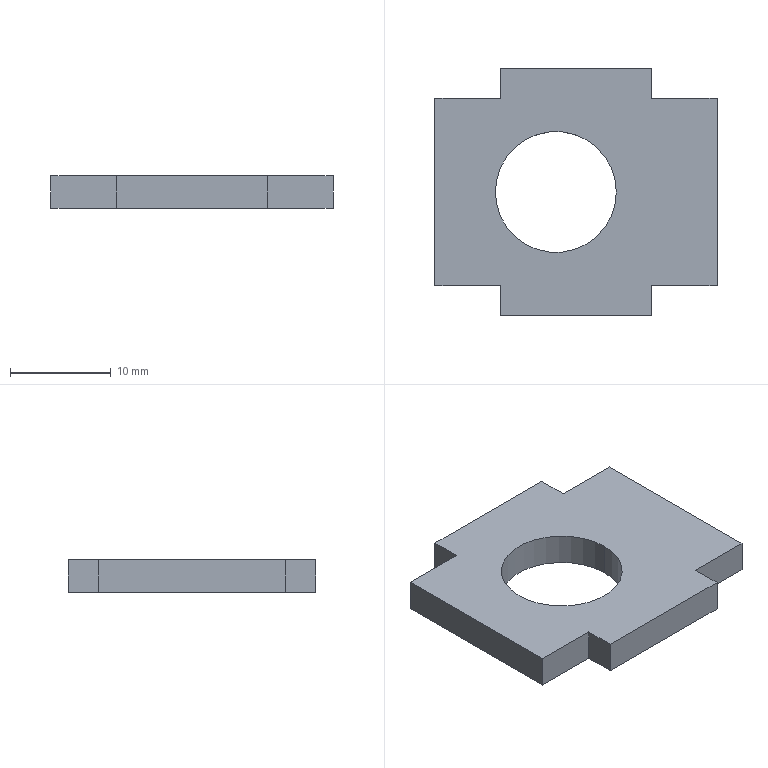Part | SolidWorks | features FlatPattern 1, SMBaseFlange 1, SheetMetal 1 | 1 solid | 16 faces | box 28 x 24.6 x 3.2 mm | volume 1593 mm3 | plane 14 | cylinder 2 | commonest cylinder face diameters 12 x2
STEP:
#1=CARTESIAN_POINT('',(213.,12.5,-3.2));
#2=VERTEX_POINT('',#1);
#3=CARTESIAN_POINT('',(225.,12.5,-3.2));
#4=VERTEX_POINT('',#3);
#5=CARTESIAN_POINT('',(219.,12.5,-3.2));
#6=DIRECTION('',(0.,0.,1.));
#7=DIRECTION('',(1.,0.,0.));
#8=AXIS2_PLACEMENT_3D('',#5,#6,#7);
#9=CIRCLE('',#8,6.);
#10=EDGE_CURVE('',#2,#4,#9,.T.);
#11=ORIENTED_EDGE('',*,*,#10,.F.);
#12=CARTESIAN_POINT('',(213.,12.5,0.));
#13=VERTEX_POINT('',#12);
#14=CARTESIAN_POINT('',(213.,12.5,-3.2));
#15=DIRECTION('',(0.,0.,1.));
#16=VECTOR('',#15,1000.);
#17=LINE('',#14,#16);
#18=EDGE_CURVE('',#2,#13,#17,.T.);
#19=ORIENTED_EDGE('',*,*,#18,.T.);
#20=CARTESIAN_POINT('',(225.,12.5,0.));
#21=VERTEX_POINT('',#20);
#22=CARTESIAN_POINT('',(219.,12.5,0.));
#23=DIRECTION('',(0.,0.,1.));
#24=DIRECTION('',(1.,0.,0.));
#25=AXIS2_PLACEMENT_3D('',#22,#23,#24);
#26=CIRCLE('',#25,6.);
#27=EDGE_CURVE('',#13,#21,#26,.T.);
#28=ORIENTED_EDGE('',*,*,#27,.T.);
#29=CARTESIAN_POINT('',(225.,12.5,-3.2));
#30=DIRECTION('',(0.,0.,1.));
#31=VECTOR('',#30,1000.);
#32=LINE('',#29,#31);
#33=EDGE_CURVE('',#4,#21,#32,.T.);
#34=ORIENTED_EDGE('',*,*,#33,.F.);
#35=EDGE_LOOP('',(#11,#19,#28,#34));
#36=FACE_OUTER_BOUND('',#35,.T.);
#37=CARTESIAN_POINT('',(219.,12.5,-3.2));
#38=DIRECTION('',(0.,0.,1.));
#39=DIRECTION('',(1.,0.,0.));
#40=AXIS2_PLACEMENT_3D('',#37,#38,#39);
#41=CYLINDRICAL_SURFACE('',#40,6.);
#42=ADVANCED_FACE('',(#36),#41,.F.);
#43=CARTESIAN_POINT('',(207.,21.8,0.));
#44=VERTEX_POINT('',#43);
#45=CARTESIAN_POINT('',(207.,3.2,0.));
#46=VERTEX_POINT('',#45);
#47=CARTESIAN_POINT('',(207.,3.2,0.));
#48=DIRECTION('',(0.,-1.,0.));
#49=VECTOR('',#48,1000.);
#50=LINE('',#47,#49);
#51=EDGE_CURVE('',#44,#46,#50,.T.);
#52=ORIENTED_EDGE('',*,*,#51,.F.);
#53=CARTESIAN_POINT('',(207.,21.8,-3.2));
#54=VERTEX_POINT('',#53);
#55=CARTESIAN_POINT('',(207.,21.8,-3.2));
#56=DIRECTION('',(0.,0.,1.));
#57=VECTOR('',#56,1000.);
#58=LINE('',#55,#57);
#59=EDGE_CURVE('',#54,#44,#58,.T.);
#60=ORIENTED_EDGE('',*,*,#59,.F.);
#61=CARTESIAN_POINT('',(207.,3.2,-3.2));
#62=VERTEX_POINT('',#61);
#63=CARTESIAN_POINT('',(207.,3.2,-3.2));
#64=DIRECTION('',(0.,-1.,0.));
#65=VECTOR('',#64,1000.);
#66=LINE('',#63,#65);
#67=EDGE_CURVE('',#54,#62,#66,.T.);
#68=ORIENTED_EDGE('',*,*,#67,.T.);
#69=CARTESIAN_POINT('',(207.,3.2,-3.2));
#70=DIRECTION('',(0.,0.,1.));
#71=VECTOR('',#70,1000.);
#72=LINE('',#69,#71);
#73=EDGE_CURVE('',#62,#46,#72,.T.);
#74=ORIENTED_EDGE('',*,*,#73,.T.);
#75=EDGE_LOOP('',(#52,#60,#68,#74));
#76=FACE_OUTER_BOUND('',#75,.T.);
#77=CARTESIAN_POINT('',(207.,3.2,-3.2));
#78=DIRECTION('',(-1.,0.,0.));
#79=DIRECTION('',(0.,0.,1.));
#80=AXIS2_PLACEMENT_3D('',#77,#78,#79);
#81=PLANE('',#80);
#82=ADVANCED_FACE('',(#76),#81,.T.);
#83=CARTESIAN_POINT('',(213.5,21.8,0.));
#84=VERTEX_POINT('',#83);
#85=CARTESIAN_POINT('',(207.,21.8,0.));
#86=DIRECTION('',(-1.,0.,0.));
#87=VECTOR('',#86,1000.);
#88=LINE('',#85,#87);
#89=EDGE_CURVE('',#84,#44,#88,.T.);
#90=ORIENTED_EDGE('',*,*,#89,.F.);
#91=CARTESIAN_POINT('',(213.5,21.8,-3.2));
#92=VERTEX_POINT('',#91);
#93=CARTESIAN_POINT('',(213.5,21.8,-3.2));
#94=DIRECTION('',(0.,0.,1.));
#95=VECTOR('',#94,1000.);
#96=LINE('',#93,#95);
#97=EDGE_CURVE('',#92,#84,#96,.T.);
#98=ORIENTED_EDGE('',*,*,#97,.F.);
#99=CARTESIAN_POINT('',(207.,21.8,-3.2));
#100=DIRECTION('',(-1.,0.,0.));
#101=VECTOR('',#100,1000.);
#102=LINE('',#99,#101);
#103=EDGE_CURVE('',#92,#54,#102,.T.);
#104=ORIENTED_EDGE('',*,*,#103,.T.);
#105=ORIENTED_EDGE('',*,*,#59,.T.);
#106=EDGE_LOOP('',(#90,#98,#104,#105));
#107=FACE_OUTER_BOUND('',#106,.T.);
#108=CARTESIAN_POINT('',(207.,21.8,-3.2));
#109=DIRECTION('',(0.,1.,0.));
#110=DIRECTION('',(0.,0.,1.));
#111=AXIS2_PLACEMENT_3D('',#108,#109,#110);
#112=PLANE('',#111);
#113=ADVANCED_FACE('',(#107),#112,.T.);
#114=CARTESIAN_POINT('',(213.5,24.8,0.));
#115=VERTEX_POINT('',#114);
#116=CARTESIAN_POINT('',(213.5,21.8,0.));
#117=DIRECTION('',(0.,-1.,0.));
#118=VECTOR('',#117,1000.);
#119=LINE('',#116,#118);
#120=EDGE_CURVE('',#115,#84,#119,.T.);
#121=ORIENTED_EDGE('',*,*,#120,.F.);
#122=CARTESIAN_POINT('',(213.5,24.8,-3.2));
#123=VERTEX_POINT('',#122);
#124=CARTESIAN_POINT('',(213.5,24.8,-3.2));
#125=DIRECTION('',(0.,0.,1.));
#126=VECTOR('',#125,1000.);
#127=LINE('',#124,#126);
#128=EDGE_CURVE('',#123,#115,#127,.T.);
#129=ORIENTED_EDGE('',*,*,#128,.F.);
#130=CARTESIAN_POINT('',(213.5,21.8,-3.2));
#131=DIRECTION('',(0.,-1.,0.));
#132=VECTOR('',#131,1000.);
#133=LINE('',#130,#132);
#134=EDGE_CURVE('',#123,#92,#133,.T.);
#135=ORIENTED_EDGE('',*,*,#134,.T.);
#136=ORIENTED_EDGE('',*,*,#97,.T.);
#137=EDGE_LOOP('',(#121,#129,#135,#136));
#138=FACE_OUTER_BOUND('',#137,.T.);
#139=CARTESIAN_POINT('',(213.5,21.8,-3.2));
#140=DIRECTION('',(-1.,0.,0.));
#141=DIRECTION('',(0.,0.,1.));
#142=AXIS2_PLACEMENT_3D('',#139,#140,#141);
#143=PLANE('',#142);
#144=ADVANCED_FACE('',(#138),#143,.T.);
#145=CARTESIAN_POINT('',(228.5,24.8,0.));
#146=VERTEX_POINT('',#145);
#147=CARTESIAN_POINT('',(213.5,24.8,0.));
#148=DIRECTION('',(-1.,0.,0.));
#149=VECTOR('',#148,1000.);
#150=LINE('',#147,#149);
#151=EDGE_CURVE('',#146,#115,#150,.T.);
#152=ORIENTED_EDGE('',*,*,#151,.F.);
#153=CARTESIAN_POINT('',(228.5,24.8,-3.2));
#154=VERTEX_POINT('',#153);
#155=CARTESIAN_POINT('',(228.5,24.8,-3.2));
#156=DIRECTION('',(0.,0.,1.));
#157=VECTOR('',#156,1000.);
#158=LINE('',#155,#157);
#159=EDGE_CURVE('',#154,#146,#158,.T.);
#160=ORIENTED_EDGE('',*,*,#159,.F.);
#161=CARTESIAN_POINT('',(213.5,24.8,-3.2));
#162=DIRECTION('',(-1.,0.,0.));
#163=VECTOR('',#162,1000.);
#164=LINE('',#161,#163);
#165=EDGE_CURVE('',#154,#123,#164,.T.);
#166=ORIENTED_EDGE('',*,*,#165,.T.);
#167=ORIENTED_EDGE('',*,*,#128,.T.);
#168=EDGE_LOOP('',(#152,#160,#166,#167));
#169=FACE_OUTER_BOUND('',#168,.T.);
#170=CARTESIAN_POINT('',(213.5,24.8,-3.2));
#171=DIRECTION('',(0.,1.,0.));
#172=DIRECTION('',(0.,0.,1.));
#173=AXIS2_PLACEMENT_3D('',#170,#171,#172);
#174=PLANE('',#173);
#175=ADVANCED_FACE('',(#169),#174,.T.);
#176=CARTESIAN_POINT('',(228.5,21.8,0.));
#177=VERTEX_POINT('',#176);
#178=CARTESIAN_POINT('',(228.5,24.8,0.));
#179=DIRECTION('',(0.,1.,0.));
#180=VECTOR('',#179,1000.);
#181=LINE('',#178,#180);
#182=EDGE_CURVE('',#177,#146,#181,.T.);
#183=ORIENTED_EDGE('',*,*,#182,.F.);
#184=CARTESIAN_POINT('',(228.5,21.8,-3.2));
#185=VERTEX_POINT('',#184);
#186=CARTESIAN_POINT('',(228.5,21.8,-3.2));
#187=DIRECTION('',(0.,0.,1.));
#188=VECTOR('',#187,1000.);
#189=LINE('',#186,#188);
#190=EDGE_CURVE('',#185,#177,#189,.T.);
#191=ORIENTED_EDGE('',*,*,#190,.F.);
#192=CARTESIAN_POINT('',(228.5,24.8,-3.2));
#193=DIRECTION('',(0.,1.,0.));
#194=VECTOR('',#193,1000.);
#195=LINE('',#192,#194);
#196=EDGE_CURVE('',#185,#154,#195,.T.);
#197=ORIENTED_EDGE('',*,*,#196,.T.);
#198=ORIENTED_EDGE('',*,*,#159,.T.);
#199=EDGE_LOOP('',(#183,#191,#197,#198));
#200=FACE_OUTER_BOUND('',#199,.T.);
#201=CARTESIAN_POINT('',(228.5,24.8,-3.2));
#202=DIRECTION('',(1.,0.,0.));
#203=DIRECTION('',(0.,0.,-1.));
#204=AXIS2_PLACEMENT_3D('',#201,#202,#203);
#205=PLANE('',#204);
#206=ADVANCED_FACE('',(#200),#205,.T.);
#207=CARTESIAN_POINT('',(235.,21.8,0.));
#208=VERTEX_POINT('',#207);
#209=CARTESIAN_POINT('',(228.5,21.8,0.));
#210=DIRECTION('',(-1.,0.,0.));
#211=VECTOR('',#210,1000.);
#212=LINE('',#209,#211);
#213=EDGE_CURVE('',#208,#177,#212,.T.);
#214=ORIENTED_EDGE('',*,*,#213,.F.);
#215=CARTESIAN_POINT('',(235.,21.8,-3.2));
#216=VERTEX_POINT('',#215);
#217=CARTESIAN_POINT('',(235.,21.8,-3.2));
#218=DIRECTION('',(0.,0.,1.));
#219=VECTOR('',#218,1000.);
#220=LINE('',#217,#219);
#221=EDGE_CURVE('',#216,#208,#220,.T.);
#222=ORIENTED_EDGE('',*,*,#221,.F.);
#223=CARTESIAN_POINT('',(228.5,21.8,-3.2));
#224=DIRECTION('',(-1.,0.,0.));
#225=VECTOR('',#224,1000.);
#226=LINE('',#223,#225);
#227=EDGE_CURVE('',#216,#185,#226,.T.);
#228=ORIENTED_EDGE('',*,*,#227,.T.);
#229=ORIENTED_EDGE('',*,*,#190,.T.);
#230=EDGE_LOOP('',(#214,#222,#228,#229));
#231=FACE_OUTER_BOUND('',#230,.T.);
#232=CARTESIAN_POINT('',(228.5,21.8,-3.2));
#233=DIRECTION('',(0.,1.,0.));
#234=DIRECTION('',(0.,0.,1.));
#235=AXIS2_PLACEMENT_3D('',#232,#233,#234);
#236=PLANE('',#235);
#237=ADVANCED_FACE('',(#231),#236,.T.);
#238=CARTESIAN_POINT('',(235.,3.2,0.));
#239=VERTEX_POINT('',#238);
#240=CARTESIAN_POINT('',(235.,3.2,0.));
#241=DIRECTION('',(0.,1.,0.));
#242=VECTOR('',#241,1000.);
#243=LINE('',#240,#242);
#244=EDGE_CURVE('',#239,#208,#243,.T.);
#245=ORIENTED_EDGE('',*,*,#244,.F.);
#246=CARTESIAN_POINT('',(235.,3.2,-3.2));
#247=VERTEX_POINT('',#246);
#248=CARTESIAN_POINT('',(235.,3.2,-3.2));
#249=DIRECTION('',(0.,0.,1.));
#250=VECTOR('',#249,1000.);
#251=LINE('',#248,#250);
#252=EDGE_CURVE('',#247,#239,#251,.T.);
#253=ORIENTED_EDGE('',*,*,#252,.F.);
#254=CARTESIAN_POINT('',(235.,3.2,-3.2));
#255=DIRECTION('',(0.,1.,0.));
#256=VECTOR('',#255,1000.);
#257=LINE('',#254,#256);
#258=EDGE_CURVE('',#247,#216,#257,.T.);
#259=ORIENTED_EDGE('',*,*,#258,.T.);
#260=ORIENTED_EDGE('',*,*,#221,.T.);
#261=EDGE_LOOP('',(#245,#253,#259,#260));
#262=FACE_OUTER_BOUND('',#261,.T.);
#263=CARTESIAN_POINT('',(235.,3.2,-3.2));
#264=DIRECTION('',(1.,0.,0.));
#265=DIRECTION('',(0.,0.,-1.));
#266=AXIS2_PLACEMENT_3D('',#263,#264,#265);
#267=PLANE('',#266);
#268=ADVANCED_FACE('',(#262),#267,.T.);
#269=CARTESIAN_POINT('',(228.5,3.2,0.));
#270=VERTEX_POINT('',#269);
#271=CARTESIAN_POINT('',(228.5,3.2,0.));
#272=DIRECTION('',(1.,0.,0.));
#273=VECTOR('',#272,1000.);
#274=LINE('',#271,#273);
#275=EDGE_CURVE('',#270,#239,#274,.T.);
#276=ORIENTED_EDGE('',*,*,#275,.F.);
#277=CARTESIAN_POINT('',(228.5,3.2,-3.2));
#278=VERTEX_POINT('',#277);
#279=CARTESIAN_POINT('',(228.5,3.2,-3.2));
#280=DIRECTION('',(0.,0.,1.));
#281=VECTOR('',#280,1000.);
#282=LINE('',#279,#281);
#283=EDGE_CURVE('',#278,#270,#282,.T.);
#284=ORIENTED_EDGE('',*,*,#283,.F.);
#285=CARTESIAN_POINT('',(228.5,3.2,-3.2));
#286=DIRECTION('',(1.,0.,0.));
#287=VECTOR('',#286,1000.);
#288=LINE('',#285,#287);
#289=EDGE_CURVE('',#278,#247,#288,.T.);
#290=ORIENTED_EDGE('',*,*,#289,.T.);
#291=ORIENTED_EDGE('',*,*,#252,.T.);
#292=EDGE_LOOP('',(#276,#284,#290,#291));
#293=FACE_OUTER_BOUND('',#292,.T.);
#294=CARTESIAN_POINT('',(228.5,3.2,-3.2));
#295=DIRECTION('',(0.,-1.,0.));
#296=DIRECTION('',(0.,0.,-1.));
#297=AXIS2_PLACEMENT_3D('',#294,#295,#296);
#298=PLANE('',#297);
#299=ADVANCED_FACE('',(#293),#298,.T.);
#300=CARTESIAN_POINT('',(228.5,0.2,0.));
#301=VERTEX_POINT('',#300);
#302=CARTESIAN_POINT('',(228.5,0.2,0.));
#303=DIRECTION('',(0.,1.,0.));
#304=VECTOR('',#303,1000.);
#305=LINE('',#302,#304);
#306=EDGE_CURVE('',#301,#270,#305,.T.);
#307=ORIENTED_EDGE('',*,*,#306,.F.);
#308=CARTESIAN_POINT('',(228.5,0.2,-3.2));
#309=VERTEX_POINT('',#308);
#310=CARTESIAN_POINT('',(228.5,0.2,-3.2));
#311=DIRECTION('',(0.,0.,1.));
#312=VECTOR('',#311,1000.);
#313=LINE('',#310,#312);
#314=EDGE_CURVE('',#309,#301,#313,.T.);
#315=ORIENTED_EDGE('',*,*,#314,.F.);
#316=CARTESIAN_POINT('',(228.5,0.2,-3.2));
#317=DIRECTION('',(0.,1.,0.));
#318=VECTOR('',#317,1000.);
#319=LINE('',#316,#318);
#320=EDGE_CURVE('',#309,#278,#319,.T.);
#321=ORIENTED_EDGE('',*,*,#320,.T.);
#322=ORIENTED_EDGE('',*,*,#283,.T.);
#323=EDGE_LOOP('',(#307,#315,#321,#322));
#324=FACE_OUTER_BOUND('',#323,.T.);
#325=CARTESIAN_POINT('',(228.5,0.2,-3.2));
#326=DIRECTION('',(1.,0.,0.));
#327=DIRECTION('',(0.,0.,-1.));
#328=AXIS2_PLACEMENT_3D('',#325,#326,#327);
#329=PLANE('',#328);
#330=ADVANCED_FACE('',(#324),#329,.T.);
#331=CARTESIAN_POINT('',(213.5,0.2,0.));
#332=VERTEX_POINT('',#331);
#333=CARTESIAN_POINT('',(213.5,0.2,0.));
#334=DIRECTION('',(1.,0.,0.));
#335=VECTOR('',#334,1000.);
#336=LINE('',#333,#335);
#337=EDGE_CURVE('',#332,#301,#336,.T.);
#338=ORIENTED_EDGE('',*,*,#337,.F.);
#339=CARTESIAN_POINT('',(213.5,0.2,-3.2));
#340=VERTEX_POINT('',#339);
#341=CARTESIAN_POINT('',(213.5,0.2,-3.2));
#342=DIRECTION('',(0.,0.,1.));
#343=VECTOR('',#342,1000.);
#344=LINE('',#341,#343);
#345=EDGE_CURVE('',#340,#332,#344,.T.);
#346=ORIENTED_EDGE('',*,*,#345,.F.);
#347=CARTESIAN_POINT('',(213.5,0.2,-3.2));
#348=DIRECTION('',(1.,0.,0.));
#349=VECTOR('',#348,1000.);
#350=LINE('',#347,#349);
#351=EDGE_CURVE('',#340,#309,#350,.T.);
#352=ORIENTED_EDGE('',*,*,#351,.T.);
#353=ORIENTED_EDGE('',*,*,#314,.T.);
#354=EDGE_LOOP('',(#338,#346,#352,#353));
#355=FACE_OUTER_BOUND('',#354,.T.);
#356=CARTESIAN_POINT('',(213.5,0.2,-3.2));
#357=DIRECTION('',(0.,-1.,0.));
#358=DIRECTION('',(0.,0.,-1.));
#359=AXIS2_PLACEMENT_3D('',#356,#357,#358);
#360=PLANE('',#359);
#361=ADVANCED_FACE('',(#355),#360,.T.);
#362=CARTESIAN_POINT('',(213.5,3.2,0.));
#363=VERTEX_POINT('',#362);
#364=CARTESIAN_POINT('',(213.5,3.2,0.));
#365=DIRECTION('',(0.,-1.,0.));
#366=VECTOR('',#365,1000.);
#367=LINE('',#364,#366);
#368=EDGE_CURVE('',#363,#332,#367,.T.);
#369=ORIENTED_EDGE('',*,*,#368,.F.);
#370=CARTESIAN_POINT('',(213.5,3.2,-3.2));
#371=VERTEX_POINT('',#370);
#372=CARTESIAN_POINT('',(213.5,3.2,-3.2));
#373=DIRECTION('',(0.,0.,1.));
#374=VECTOR('',#373,1000.);
#375=LINE('',#372,#374);
#376=EDGE_CURVE('',#371,#363,#375,.T.);
#377=ORIENTED_EDGE('',*,*,#376,.F.);
#378=CARTESIAN_POINT('',(213.5,3.2,-3.2));
#379=DIRECTION('',(0.,-1.,0.));
#380=VECTOR('',#379,1000.);
#381=LINE('',#378,#380);
#382=EDGE_CURVE('',#371,#340,#381,.T.);
#383=ORIENTED_EDGE('',*,*,#382,.T.);
#384=ORIENTED_EDGE('',*,*,#345,.T.);
#385=EDGE_LOOP('',(#369,#377,#383,#384));
#386=FACE_OUTER_BOUND('',#385,.T.);
#387=CARTESIAN_POINT('',(213.5,3.2,-3.2));
#388=DIRECTION('',(-1.,0.,0.));
#389=DIRECTION('',(0.,0.,1.));
#390=AXIS2_PLACEMENT_3D('',#387,#388,#389);
#391=PLANE('',#390);
#392=ADVANCED_FACE('',(#386),#391,.T.);
#393=CARTESIAN_POINT('',(207.,3.2,0.));
#394=DIRECTION('',(1.,0.,0.));
#395=VECTOR('',#394,1000.);
#396=LINE('',#393,#395);
#397=EDGE_CURVE('',#46,#363,#396,.T.);
#398=ORIENTED_EDGE('',*,*,#397,.F.);
#399=ORIENTED_EDGE('',*,*,#73,.F.);
#400=CARTESIAN_POINT('',(207.,3.2,-3.2));
#401=DIRECTION('',(1.,0.,0.));
#402=VECTOR('',#401,1000.);
#403=LINE('',#400,#402);
#404=EDGE_CURVE('',#62,#371,#403,.T.);
#405=ORIENTED_EDGE('',*,*,#404,.T.);
#406=ORIENTED_EDGE('',*,*,#376,.T.);
#407=EDGE_LOOP('',(#398,#399,#405,#406));
#408=FACE_OUTER_BOUND('',#407,.T.);
#409=CARTESIAN_POINT('',(207.,3.2,-3.2));
#410=DIRECTION('',(0.,-1.,0.));
#411=DIRECTION('',(1.,0.,0.));
#412=AXIS2_PLACEMENT_3D('',#409,#410,#411);
#413=PLANE('',#412);
#414=ADVANCED_FACE('',(#408),#413,.T.);
#415=CARTESIAN_POINT('',(219.,12.5,-3.2));
#416=DIRECTION('',(0.,0.,1.));
#417=DIRECTION('',(1.,0.,0.));
#418=AXIS2_PLACEMENT_3D('',#415,#416,#417);
#419=CIRCLE('',#418,6.);
#420=EDGE_CURVE('',#4,#2,#419,.T.);
#421=ORIENTED_EDGE('',*,*,#420,.T.);
#422=ORIENTED_EDGE('',*,*,#10,.T.);
#423=EDGE_LOOP('',(#421,#422));
#424=FACE_BOUND('',#423,.T.);
#425=ORIENTED_EDGE('',*,*,#67,.F.);
#426=ORIENTED_EDGE('',*,*,#103,.F.);
#427=ORIENTED_EDGE('',*,*,#134,.F.);
#428=ORIENTED_EDGE('',*,*,#165,.F.);
#429=ORIENTED_EDGE('',*,*,#196,.F.);
#430=ORIENTED_EDGE('',*,*,#227,.F.);
#431=ORIENTED_EDGE('',*,*,#258,.F.);
#432=ORIENTED_EDGE('',*,*,#289,.F.);
#433=ORIENTED_EDGE('',*,*,#320,.F.);
#434=ORIENTED_EDGE('',*,*,#351,.F.);
#435=ORIENTED_EDGE('',*,*,#382,.F.);
#436=ORIENTED_EDGE('',*,*,#404,.F.);
#437=EDGE_LOOP('',(#425,#426,#427,#428,#429,#430,#431,#432,#433,#434,#435,#436));
#438=FACE_OUTER_BOUND('',#437,.T.);
#439=CARTESIAN_POINT('',(0.,0.,-3.2));
#440=DIRECTION('',(0.,0.,-1.));
#441=DIRECTION('',(-1.,0.,0.));
#442=AXIS2_PLACEMENT_3D('',#439,#440,#441);
#443=PLANE('',#442);
#444=ADVANCED_FACE('',(#424,#438),#443,.T.);
#445=CARTESIAN_POINT('',(219.,12.5,0.));
#446=DIRECTION('',(0.,0.,1.));
#447=DIRECTION('',(1.,0.,0.));
#448=AXIS2_PLACEMENT_3D('',#445,#446,#447);
#449=CIRCLE('',#448,6.);
#450=EDGE_CURVE('',#21,#13,#449,.T.);
#451=ORIENTED_EDGE('',*,*,#450,.F.);
#452=ORIENTED_EDGE('',*,*,#27,.F.);
#453=EDGE_LOOP('',(#451,#452));
#454=FACE_BOUND('',#453,.T.);
#455=ORIENTED_EDGE('',*,*,#51,.T.);
#456=ORIENTED_EDGE('',*,*,#397,.T.);
#457=ORIENTED_EDGE('',*,*,#368,.T.);
#458=ORIENTED_EDGE('',*,*,#337,.T.);
#459=ORIENTED_EDGE('',*,*,#306,.T.);
#460=ORIENTED_EDGE('',*,*,#275,.T.);
#461=ORIENTED_EDGE('',*,*,#244,.T.);
#462=ORIENTED_EDGE('',*,*,#213,.T.);
#463=ORIENTED_EDGE('',*,*,#182,.T.);
#464=ORIENTED_EDGE('',*,*,#151,.T.);
#465=ORIENTED_EDGE('',*,*,#120,.T.);
#466=ORIENTED_EDGE('',*,*,#89,.T.);
#467=EDGE_LOOP('',(#455,#456,#457,#458,#459,#460,#461,#462,#463,#464,#465,#466));
#468=FACE_OUTER_BOUND('',#467,.T.);
#469=CARTESIAN_POINT('',(0.,0.,0.));
#470=DIRECTION('',(0.,0.,-1.));
#471=DIRECTION('',(-1.,0.,0.));
#472=AXIS2_PLACEMENT_3D('',#469,#470,#471);
#473=PLANE('',#472);
#474=ADVANCED_FACE('',(#454,#468),#473,.F.);
#475=ORIENTED_EDGE('',*,*,#18,.F.);
#476=ORIENTED_EDGE('',*,*,#420,.F.);
#477=ORIENTED_EDGE('',*,*,#33,.T.);
#478=ORIENTED_EDGE('',*,*,#450,.T.);
#479=EDGE_LOOP('',(#475,#476,#477,#478));
#480=FACE_OUTER_BOUND('',#479,.T.);
#481=CARTESIAN_POINT('',(219.,12.5,-3.2));
#482=DIRECTION('',(0.,0.,1.));
#483=DIRECTION('',(1.,0.,0.));
#484=AXIS2_PLACEMENT_3D('',#481,#482,#483);
#485=CYLINDRICAL_SURFACE('',#484,6.);
#486=ADVANCED_FACE('',(#480),#485,.F.);
#487=CLOSED_SHELL('',(#42,#82,#113,#144,#175,#206,#237,#268,#299,#330,#361,#392,#414,#444,#474,#486));
#488=MANIFOLD_SOLID_BREP('',#487);
#489=CARTESIAN_POINT('',(0.,0.,0.));
#490=DIRECTION('',(0.,0.,1.));
#491=DIRECTION('',(1.,0.,0.));
#492=AXIS2_PLACEMENT_3D('',#489,#490,#491);
#493=(LENGTH_UNIT()NAMED_UNIT(*)SI_UNIT(.MILLI.,.METRE.));
#494=UNCERTAINTY_MEASURE_WITH_UNIT(LENGTH_MEASURE(0.00001),#493,'','');
#495=(NAMED_UNIT(*)PLANE_ANGLE_UNIT()SI_UNIT($,.RADIAN.));
#496=(NAMED_UNIT(*)SI_UNIT($,.STERADIAN.)SOLID_ANGLE_UNIT());
#497=(GEOMETRIC_REPRESENTATION_CONTEXT(3)GLOBAL_UNCERTAINTY_ASSIGNED_CONTEXT((#494))GLOBAL_UNIT_ASSIGNED_CONTEXT((#493,#495,#496))REPRESENTATION_CONTEXT('',''));
#498=ADVANCED_BREP_SHAPE_REPRESENTATION('',(#488,#492),#497);